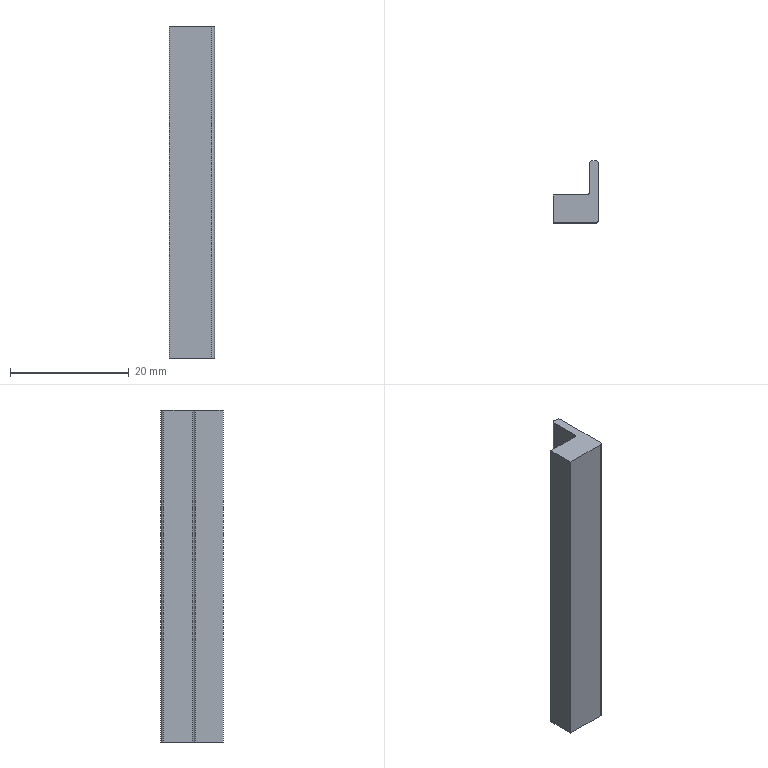Part | NX | features BREP 2 | 2 solids | 24 faces | box 7.6 x 10.5 x 56 mm | volume 4963 mm3 | plane 16 | cylinder 8 | commonest cylinder face diameters 1 x8
STEP:
#1=CARTESIAN_POINT('',(2.3,-0.05,-4.));
#2=VERTEX_POINT('',#1);
#3=CARTESIAN_POINT('',(2.3,-0.05,52.));
#4=VERTEX_POINT('',#3);
#5=CARTESIAN_POINT('',(2.3,-0.05,0.));
#6=DIRECTION('',(0.,0.,1.));
#7=VECTOR('',#6,1000.);
#8=LINE('',#5,#7);
#9=EDGE_CURVE('',#2,#4,#8,.T.);
#10=ORIENTED_EDGE('',*,*,#9,.T.);
#11=CARTESIAN_POINT('',(2.3,4.75,52.));
#12=VERTEX_POINT('',#11);
#13=CARTESIAN_POINT('',(2.3,4.728,52.));
#14=DIRECTION('',(0.,-1.,0.));
#15=VECTOR('',#14,1000.);
#16=LINE('',#13,#15);
#17=EDGE_CURVE('',#12,#4,#16,.T.);
#18=ORIENTED_EDGE('',*,*,#17,.F.);
#19=CARTESIAN_POINT('',(2.3,4.75,-4.));
#20=VERTEX_POINT('',#19);
#21=CARTESIAN_POINT('',(2.3,4.75,0.));
#22=DIRECTION('',(0.,0.,1.));
#23=VECTOR('',#22,1000.);
#24=LINE('',#21,#23);
#25=EDGE_CURVE('',#20,#12,#24,.T.);
#26=ORIENTED_EDGE('',*,*,#25,.F.);
#27=CARTESIAN_POINT('',(2.3,4.728,-4.));
#28=DIRECTION('',(0.,-1.,0.));
#29=VECTOR('',#28,1000.);
#30=LINE('',#27,#29);
#31=EDGE_CURVE('',#20,#2,#30,.T.);
#32=ORIENTED_EDGE('',*,*,#31,.T.);
#33=EDGE_LOOP('',(#10,#18,#26,#32));
#34=FACE_BOUND('',#33,.T.);
#35=CARTESIAN_POINT('',(2.3,-0.05,0.));
#36=DIRECTION('',(1.,0.,0.));
#37=DIRECTION('',(0.,-1.,0.));
#38=AXIS2_PLACEMENT_3D('',#35,#36,#37);
#39=PLANE('',#38);
#40=ADVANCED_FACE('',(#34),#39,.F.);
#41=ORIENTED_EDGE('',*,*,#25,.T.);
#42=CARTESIAN_POINT('',(2.8,5.25,52.));
#43=VERTEX_POINT('',#42);
#44=CARTESIAN_POINT('',(2.8,4.75,52.));
#45=DIRECTION('',(0.,0.,1.));
#46=DIRECTION('',(1.,0.,0.));
#47=AXIS2_PLACEMENT_3D('',#44,#45,#46);
#48=CIRCLE('',#47,0.5);
#49=EDGE_CURVE('',#43,#12,#48,.T.);
#50=ORIENTED_EDGE('',*,*,#49,.F.);
#51=CARTESIAN_POINT('',(2.8,5.25,-4.));
#52=VERTEX_POINT('',#51);
#53=CARTESIAN_POINT('',(2.8,5.25,0.));
#54=DIRECTION('',(0.,0.,1.));
#55=VECTOR('',#54,1000.);
#56=LINE('',#53,#55);
#57=EDGE_CURVE('',#52,#43,#56,.T.);
#58=ORIENTED_EDGE('',*,*,#57,.F.);
#59=CARTESIAN_POINT('',(2.8,4.75,-4.));
#60=DIRECTION('',(0.,0.,1.));
#61=DIRECTION('',(1.,0.,0.));
#62=AXIS2_PLACEMENT_3D('',#59,#60,#61);
#63=CIRCLE('',#62,0.5);
#64=EDGE_CURVE('',#52,#20,#63,.T.);
#65=ORIENTED_EDGE('',*,*,#64,.T.);
#66=EDGE_LOOP('',(#41,#50,#58,#65));
#67=FACE_BOUND('',#66,.T.);
#68=CARTESIAN_POINT('',(2.8,4.75,0.));
#69=DIRECTION('',(0.,0.,1.));
#70=DIRECTION('',(-1.,0.,0.));
#71=AXIS2_PLACEMENT_3D('',#68,#69,#70);
#72=CYLINDRICAL_SURFACE('',#71,0.5);
#73=ADVANCED_FACE('',(#67),#72,.T.);
#74=ORIENTED_EDGE('',*,*,#57,.T.);
#75=CARTESIAN_POINT('',(3.3,5.25,52.));
#76=VERTEX_POINT('',#75);
#77=CARTESIAN_POINT('',(5.273,5.25,52.));
#78=DIRECTION('',(-1.,0.,0.));
#79=VECTOR('',#78,1000.);
#80=LINE('',#77,#79);
#81=EDGE_CURVE('',#76,#43,#80,.T.);
#82=ORIENTED_EDGE('',*,*,#81,.F.);
#83=CARTESIAN_POINT('',(3.3,5.25,-4.));
#84=VERTEX_POINT('',#83);
#85=CARTESIAN_POINT('',(3.3,5.25,0.));
#86=DIRECTION('',(0.,0.,1.));
#87=VECTOR('',#86,1000.);
#88=LINE('',#85,#87);
#89=EDGE_CURVE('',#84,#76,#88,.T.);
#90=ORIENTED_EDGE('',*,*,#89,.F.);
#91=CARTESIAN_POINT('',(5.273,5.25,-4.));
#92=DIRECTION('',(-1.,0.,0.));
#93=VECTOR('',#92,1000.);
#94=LINE('',#91,#93);
#95=EDGE_CURVE('',#84,#52,#94,.T.);
#96=ORIENTED_EDGE('',*,*,#95,.T.);
#97=EDGE_LOOP('',(#74,#82,#90,#96));
#98=FACE_BOUND('',#97,.T.);
#99=CARTESIAN_POINT('',(2.8,5.25,0.));
#100=DIRECTION('',(0.,-1.,0.));
#101=DIRECTION('',(-1.,0.,0.));
#102=AXIS2_PLACEMENT_3D('',#99,#100,#101);
#103=PLANE('',#102);
#104=ADVANCED_FACE('',(#98),#103,.F.);
#105=ORIENTED_EDGE('',*,*,#89,.T.);
#106=CARTESIAN_POINT('',(3.8,4.75,52.));
#107=VERTEX_POINT('',#106);
#108=CARTESIAN_POINT('',(3.3,4.75,52.));
#109=DIRECTION('',(0.,0.,1.));
#110=DIRECTION('',(1.,0.,0.));
#111=AXIS2_PLACEMENT_3D('',#108,#109,#110);
#112=CIRCLE('',#111,0.5);
#113=EDGE_CURVE('',#107,#76,#112,.T.);
#114=ORIENTED_EDGE('',*,*,#113,.F.);
#115=CARTESIAN_POINT('',(3.8,4.75,-4.));
#116=VERTEX_POINT('',#115);
#117=CARTESIAN_POINT('',(3.8,4.75,0.));
#118=DIRECTION('',(0.,0.,1.));
#119=VECTOR('',#118,1000.);
#120=LINE('',#117,#119);
#121=EDGE_CURVE('',#116,#107,#120,.T.);
#122=ORIENTED_EDGE('',*,*,#121,.F.);
#123=CARTESIAN_POINT('',(3.3,4.75,-4.));
#124=DIRECTION('',(0.,0.,1.));
#125=DIRECTION('',(1.,0.,0.));
#126=AXIS2_PLACEMENT_3D('',#123,#124,#125);
#127=CIRCLE('',#126,0.5);
#128=EDGE_CURVE('',#116,#84,#127,.T.);
#129=ORIENTED_EDGE('',*,*,#128,.T.);
#130=EDGE_LOOP('',(#105,#114,#122,#129));
#131=FACE_BOUND('',#130,.T.);
#132=CARTESIAN_POINT('',(3.3,4.75,0.));
#133=DIRECTION('',(0.,0.,1.));
#134=DIRECTION('',(-1.,0.,0.));
#135=AXIS2_PLACEMENT_3D('',#132,#133,#134);
#136=CYLINDRICAL_SURFACE('',#135,0.5);
#137=ADVANCED_FACE('',(#131),#136,.T.);
#138=ORIENTED_EDGE('',*,*,#121,.T.);
#139=CARTESIAN_POINT('',(3.8,-4.75,52.));
#140=VERTEX_POINT('',#139);
#141=CARTESIAN_POINT('',(3.8,4.728,52.));
#142=DIRECTION('',(0.,1.,0.));
#143=VECTOR('',#142,1000.);
#144=LINE('',#141,#143);
#145=EDGE_CURVE('',#140,#107,#144,.T.);
#146=ORIENTED_EDGE('',*,*,#145,.F.);
#147=CARTESIAN_POINT('',(3.8,-4.75,-4.));
#148=VERTEX_POINT('',#147);
#149=CARTESIAN_POINT('',(3.8,-4.75,0.));
#150=DIRECTION('',(0.,0.,1.));
#151=VECTOR('',#150,1000.);
#152=LINE('',#149,#151);
#153=EDGE_CURVE('',#148,#140,#152,.T.);
#154=ORIENTED_EDGE('',*,*,#153,.F.);
#155=CARTESIAN_POINT('',(3.8,4.728,-4.));
#156=DIRECTION('',(0.,1.,0.));
#157=VECTOR('',#156,1000.);
#158=LINE('',#155,#157);
#159=EDGE_CURVE('',#148,#116,#158,.T.);
#160=ORIENTED_EDGE('',*,*,#159,.T.);
#161=EDGE_LOOP('',(#138,#146,#154,#160));
#162=FACE_BOUND('',#161,.T.);
#163=CARTESIAN_POINT('',(3.8,4.75,0.));
#164=DIRECTION('',(-1.,0.,0.));
#165=DIRECTION('',(0.,1.,0.));
#166=AXIS2_PLACEMENT_3D('',#163,#164,#165);
#167=PLANE('',#166);
#168=ADVANCED_FACE('',(#162),#167,.F.);
#169=ORIENTED_EDGE('',*,*,#153,.T.);
#170=CARTESIAN_POINT('',(3.3,-5.25,52.));
#171=VERTEX_POINT('',#170);
#172=CARTESIAN_POINT('',(3.3,-4.75,52.));
#173=DIRECTION('',(0.,0.,1.));
#174=DIRECTION('',(1.,0.,0.));
#175=AXIS2_PLACEMENT_3D('',#172,#173,#174);
#176=CIRCLE('',#175,0.5);
#177=EDGE_CURVE('',#171,#140,#176,.T.);
#178=ORIENTED_EDGE('',*,*,#177,.F.);
#179=CARTESIAN_POINT('',(3.3,-5.25,-4.));
#180=VERTEX_POINT('',#179);
#181=CARTESIAN_POINT('',(3.3,-5.25,0.));
#182=DIRECTION('',(0.,0.,1.));
#183=VECTOR('',#182,1000.);
#184=LINE('',#181,#183);
#185=EDGE_CURVE('',#180,#171,#184,.T.);
#186=ORIENTED_EDGE('',*,*,#185,.F.);
#187=CARTESIAN_POINT('',(3.3,-4.75,-4.));
#188=DIRECTION('',(0.,0.,1.));
#189=DIRECTION('',(1.,0.,0.));
#190=AXIS2_PLACEMENT_3D('',#187,#188,#189);
#191=CIRCLE('',#190,0.5);
#192=EDGE_CURVE('',#180,#148,#191,.T.);
#193=ORIENTED_EDGE('',*,*,#192,.T.);
#194=EDGE_LOOP('',(#169,#178,#186,#193));
#195=FACE_BOUND('',#194,.T.);
#196=CARTESIAN_POINT('',(3.3,-4.75,0.));
#197=DIRECTION('',(0.,0.,1.));
#198=DIRECTION('',(-1.,0.,0.));
#199=AXIS2_PLACEMENT_3D('',#196,#197,#198);
#200=CYLINDRICAL_SURFACE('',#199,0.5);
#201=ADVANCED_FACE('',(#195),#200,.T.);
#202=ORIENTED_EDGE('',*,*,#185,.T.);
#203=CARTESIAN_POINT('',(-3.8,-5.25,52.));
#204=VERTEX_POINT('',#203);
#205=CARTESIAN_POINT('',(5.273,-5.25,52.));
#206=DIRECTION('',(1.,0.,0.));
#207=VECTOR('',#206,1000.);
#208=LINE('',#205,#207);
#209=EDGE_CURVE('',#204,#171,#208,.T.);
#210=ORIENTED_EDGE('',*,*,#209,.F.);
#211=CARTESIAN_POINT('',(-3.8,-5.25,-4.));
#212=VERTEX_POINT('',#211);
#213=CARTESIAN_POINT('',(-3.8,-5.25,0.));
#214=DIRECTION('',(0.,0.,1.));
#215=VECTOR('',#214,1000.);
#216=LINE('',#213,#215);
#217=EDGE_CURVE('',#212,#204,#216,.T.);
#218=ORIENTED_EDGE('',*,*,#217,.F.);
#219=CARTESIAN_POINT('',(5.273,-5.25,-4.));
#220=DIRECTION('',(1.,0.,0.));
#221=VECTOR('',#220,1000.);
#222=LINE('',#219,#221);
#223=EDGE_CURVE('',#212,#180,#222,.T.);
#224=ORIENTED_EDGE('',*,*,#223,.T.);
#225=EDGE_LOOP('',(#202,#210,#218,#224));
#226=FACE_BOUND('',#225,.T.);
#227=CARTESIAN_POINT('',(3.3,-5.25,0.));
#228=DIRECTION('',(0.,1.,0.));
#229=DIRECTION('',(1.,0.,0.));
#230=AXIS2_PLACEMENT_3D('',#227,#228,#229);
#231=PLANE('',#230);
#232=ADVANCED_FACE('',(#226),#231,.F.);
#233=ORIENTED_EDGE('',*,*,#217,.T.);
#234=CARTESIAN_POINT('',(-3.8,-0.55,52.));
#235=VERTEX_POINT('',#234);
#236=CARTESIAN_POINT('',(-3.8,4.728,52.));
#237=DIRECTION('',(0.,-1.,0.));
#238=VECTOR('',#237,1000.);
#239=LINE('',#236,#238);
#240=EDGE_CURVE('',#235,#204,#239,.T.);
#241=ORIENTED_EDGE('',*,*,#240,.F.);
#242=CARTESIAN_POINT('',(-3.8,-0.55,-4.));
#243=VERTEX_POINT('',#242);
#244=CARTESIAN_POINT('',(-3.8,-0.55,0.));
#245=DIRECTION('',(0.,0.,1.));
#246=VECTOR('',#245,1000.);
#247=LINE('',#244,#246);
#248=EDGE_CURVE('',#243,#235,#247,.T.);
#249=ORIENTED_EDGE('',*,*,#248,.F.);
#250=CARTESIAN_POINT('',(-3.8,4.728,-4.));
#251=DIRECTION('',(0.,-1.,0.));
#252=VECTOR('',#251,1000.);
#253=LINE('',#250,#252);
#254=EDGE_CURVE('',#243,#212,#253,.T.);
#255=ORIENTED_EDGE('',*,*,#254,.T.);
#256=EDGE_LOOP('',(#233,#241,#249,#255));
#257=FACE_BOUND('',#256,.T.);
#258=CARTESIAN_POINT('',(-3.8,4.728,0.));
#259=DIRECTION('',(-1.,0.,0.));
#260=DIRECTION('',(0.,1.,0.));
#261=AXIS2_PLACEMENT_3D('',#258,#259,#260);
#262=PLANE('',#261);
#263=ADVANCED_FACE('',(#257),#262,.T.);
#264=ORIENTED_EDGE('',*,*,#248,.T.);
#265=CARTESIAN_POINT('',(1.8,-0.55,52.));
#266=VERTEX_POINT('',#265);
#267=CARTESIAN_POINT('',(5.273,-0.55,52.));
#268=DIRECTION('',(-1.,0.,0.));
#269=VECTOR('',#268,1000.);
#270=LINE('',#267,#269);
#271=EDGE_CURVE('',#266,#235,#270,.T.);
#272=ORIENTED_EDGE('',*,*,#271,.F.);
#273=CARTESIAN_POINT('',(1.8,-0.55,-4.));
#274=VERTEX_POINT('',#273);
#275=CARTESIAN_POINT('',(1.8,-0.55,0.));
#276=DIRECTION('',(0.,0.,1.));
#277=VECTOR('',#276,1000.);
#278=LINE('',#275,#277);
#279=EDGE_CURVE('',#274,#266,#278,.T.);
#280=ORIENTED_EDGE('',*,*,#279,.F.);
#281=CARTESIAN_POINT('',(5.273,-0.55,-4.));
#282=DIRECTION('',(-1.,0.,0.));
#283=VECTOR('',#282,1000.);
#284=LINE('',#281,#283);
#285=EDGE_CURVE('',#274,#243,#284,.T.);
#286=ORIENTED_EDGE('',*,*,#285,.T.);
#287=EDGE_LOOP('',(#264,#272,#280,#286));
#288=FACE_BOUND('',#287,.T.);
#289=CARTESIAN_POINT('',(-9.777,-0.55,0.));
#290=DIRECTION('',(0.,-1.,0.));
#291=DIRECTION('',(-1.,0.,0.));
#292=AXIS2_PLACEMENT_3D('',#289,#290,#291);
#293=PLANE('',#292);
#294=ADVANCED_FACE('',(#288),#293,.F.);
#295=CARTESIAN_POINT('',(1.8,-0.05,-4.));
#296=DIRECTION('',(0.,0.,-1.));
#297=DIRECTION('',(1.,0.,0.));
#298=AXIS2_PLACEMENT_3D('',#295,#296,#297);
#299=CIRCLE('',#298,0.5);
#300=EDGE_CURVE('',#2,#274,#299,.T.);
#301=ORIENTED_EDGE('',*,*,#300,.T.);
#302=ORIENTED_EDGE('',*,*,#279,.T.);
#303=CARTESIAN_POINT('',(1.8,-0.05,52.));
#304=DIRECTION('',(0.,0.,-1.));
#305=DIRECTION('',(1.,0.,0.));
#306=AXIS2_PLACEMENT_3D('',#303,#304,#305);
#307=CIRCLE('',#306,0.5);
#308=EDGE_CURVE('',#4,#266,#307,.T.);
#309=ORIENTED_EDGE('',*,*,#308,.F.);
#310=ORIENTED_EDGE('',*,*,#9,.F.);
#311=EDGE_LOOP('',(#301,#302,#309,#310));
#312=FACE_BOUND('',#311,.T.);
#313=CARTESIAN_POINT('',(1.8,-0.05,0.));
#314=DIRECTION('',(0.,0.,1.));
#315=DIRECTION('',(-1.,0.,0.));
#316=AXIS2_PLACEMENT_3D('',#313,#314,#315);
#317=CYLINDRICAL_SURFACE('',#316,0.5);
#318=ADVANCED_FACE('',(#312),#317,.F.);
#319=ORIENTED_EDGE('',*,*,#271,.T.);
#320=ORIENTED_EDGE('',*,*,#240,.T.);
#321=ORIENTED_EDGE('',*,*,#209,.T.);
#322=ORIENTED_EDGE('',*,*,#177,.T.);
#323=ORIENTED_EDGE('',*,*,#145,.T.);
#324=ORIENTED_EDGE('',*,*,#113,.T.);
#325=ORIENTED_EDGE('',*,*,#81,.T.);
#326=ORIENTED_EDGE('',*,*,#49,.T.);
#327=ORIENTED_EDGE('',*,*,#17,.T.);
#328=ORIENTED_EDGE('',*,*,#308,.T.);
#329=EDGE_LOOP('',(#319,#320,#321,#322,#323,#324,#325,#326,#327,#328));
#330=FACE_BOUND('',#329,.T.);
#331=CARTESIAN_POINT('',(5.273,4.728,52.));
#332=DIRECTION('',(0.,0.,1.));
#333=DIRECTION('',(-1.,0.,0.));
#334=AXIS2_PLACEMENT_3D('',#331,#332,#333);
#335=PLANE('',#334);
#336=ADVANCED_FACE('',(#330),#335,.T.);
#337=ORIENTED_EDGE('',*,*,#285,.F.);
#338=ORIENTED_EDGE('',*,*,#300,.F.);
#339=ORIENTED_EDGE('',*,*,#31,.F.);
#340=ORIENTED_EDGE('',*,*,#64,.F.);
#341=ORIENTED_EDGE('',*,*,#95,.F.);
#342=ORIENTED_EDGE('',*,*,#128,.F.);
#343=ORIENTED_EDGE('',*,*,#159,.F.);
#344=ORIENTED_EDGE('',*,*,#192,.F.);
#345=ORIENTED_EDGE('',*,*,#223,.F.);
#346=ORIENTED_EDGE('',*,*,#254,.F.);
#347=EDGE_LOOP('',(#337,#338,#339,#340,#341,#342,#343,#344,#345,#346));
#348=FACE_BOUND('',#347,.T.);
#349=CARTESIAN_POINT('',(5.273,4.728,-4.));
#350=DIRECTION('',(0.,0.,1.));
#351=DIRECTION('',(-1.,0.,0.));
#352=AXIS2_PLACEMENT_3D('',#349,#350,#351);
#353=PLANE('',#352);
#354=ADVANCED_FACE('',(#348),#353,.F.);
#355=CLOSED_SHELL('',(#40,#73,#104,#137,#168,#201,#232,#263,#294,#318,#336,#354));
#356=MANIFOLD_SOLID_BREP('',#355);
#357=CARTESIAN_POINT('',(2.3,-0.05,-4.));
#358=VERTEX_POINT('',#357);
#359=CARTESIAN_POINT('',(2.3,-0.05,52.));
#360=VERTEX_POINT('',#359);
#361=CARTESIAN_POINT('',(2.3,-0.05,0.));
#362=DIRECTION('',(0.,0.,1.));
#363=VECTOR('',#362,1000.);
#364=LINE('',#361,#363);
#365=EDGE_CURVE('',#358,#360,#364,.T.);
#366=ORIENTED_EDGE('',*,*,#365,.T.);
#367=CARTESIAN_POINT('',(2.3,4.75,52.));
#368=VERTEX_POINT('',#367);
#369=CARTESIAN_POINT('',(2.3,4.728,52.));
#370=DIRECTION('',(0.,-1.,0.));
#371=VECTOR('',#370,1000.);
#372=LINE('',#369,#371);
#373=EDGE_CURVE('',#368,#360,#372,.T.);
#374=ORIENTED_EDGE('',*,*,#373,.F.);
#375=CARTESIAN_POINT('',(2.3,4.75,-4.));
#376=VERTEX_POINT('',#375);
#377=CARTESIAN_POINT('',(2.3,4.75,0.));
#378=DIRECTION('',(0.,0.,1.));
#379=VECTOR('',#378,1000.);
#380=LINE('',#377,#379);
#381=EDGE_CURVE('',#376,#368,#380,.T.);
#382=ORIENTED_EDGE('',*,*,#381,.F.);
#383=CARTESIAN_POINT('',(2.3,4.728,-4.));
#384=DIRECTION('',(0.,-1.,0.));
#385=VECTOR('',#384,1000.);
#386=LINE('',#383,#385);
#387=EDGE_CURVE('',#376,#358,#386,.T.);
#388=ORIENTED_EDGE('',*,*,#387,.T.);
#389=EDGE_LOOP('',(#366,#374,#382,#388));
#390=FACE_BOUND('',#389,.T.);
#391=CARTESIAN_POINT('',(2.3,-0.05,0.));
#392=DIRECTION('',(1.,0.,0.));
#393=DIRECTION('',(0.,-1.,0.));
#394=AXIS2_PLACEMENT_3D('',#391,#392,#393);
#395=PLANE('',#394);
#396=ADVANCED_FACE('',(#390),#395,.F.);
#397=ORIENTED_EDGE('',*,*,#381,.T.);
#398=CARTESIAN_POINT('',(2.8,5.25,52.));
#399=VERTEX_POINT('',#398);
#400=CARTESIAN_POINT('',(2.8,4.75,52.));
#401=DIRECTION('',(0.,0.,1.));
#402=DIRECTION('',(1.,0.,0.));
#403=AXIS2_PLACEMENT_3D('',#400,#401,#402);
#404=CIRCLE('',#403,0.5);
#405=EDGE_CURVE('',#399,#368,#404,.T.);
#406=ORIENTED_EDGE('',*,*,#405,.F.);
#407=CARTESIAN_POINT('',(2.8,5.25,-4.));
#408=VERTEX_POINT('',#407);
#409=CARTESIAN_POINT('',(2.8,5.25,0.));
#410=DIRECTION('',(0.,0.,1.));
#411=VECTOR('',#410,1000.);
#412=LINE('',#409,#411);
#413=EDGE_CURVE('',#408,#399,#412,.T.);
#414=ORIENTED_EDGE('',*,*,#413,.F.);
#415=CARTESIAN_POINT('',(2.8,4.75,-4.));
#416=DIRECTION('',(0.,0.,1.));
#417=DIRECTION('',(1.,0.,0.));
#418=AXIS2_PLACEMENT_3D('',#415,#416,#417);
#419=CIRCLE('',#418,0.5);
#420=EDGE_CURVE('',#408,#376,#419,.T.);
#421=ORIENTED_EDGE('',*,*,#420,.T.);
#422=EDGE_LOOP('',(#397,#406,#414,#421));
#423=FACE_BOUND('',#422,.T.);
#424=CARTESIAN_POINT('',(2.8,4.75,0.));
#425=DIRECTION('',(0.,0.,1.));
#426=DIRECTION('',(-1.,0.,0.));
#427=AXIS2_PLACEMENT_3D('',#424,#425,#426);
#428=CYLINDRICAL_SURFACE('',#427,0.5);
#429=ADVANCED_FACE('',(#423),#428,.T.);
#430=ORIENTED_EDGE('',*,*,#413,.T.);
#431=CARTESIAN_POINT('',(3.3,5.25,52.));
#432=VERTEX_POINT('',#431);
#433=CARTESIAN_POINT('',(5.273,5.25,52.));
#434=DIRECTION('',(-1.,0.,0.));
#435=VECTOR('',#434,1000.);
#436=LINE('',#433,#435);
#437=EDGE_CURVE('',#432,#399,#436,.T.);
#438=ORIENTED_EDGE('',*,*,#437,.F.);
#439=CARTESIAN_POINT('',(3.3,5.25,-4.));
#440=VERTEX_POINT('',#439);
#441=CARTESIAN_POINT('',(3.3,5.25,0.));
#442=DIRECTION('',(0.,0.,1.));
#443=VECTOR('',#442,1000.);
#444=LINE('',#441,#443);
#445=EDGE_CURVE('',#440,#432,#444,.T.);
#446=ORIENTED_EDGE('',*,*,#445,.F.);
#447=CARTESIAN_POINT('',(5.273,5.25,-4.));
#448=DIRECTION('',(-1.,0.,0.));
#449=VECTOR('',#448,1000.);
#450=LINE('',#447,#449);
#451=EDGE_CURVE('',#440,#408,#450,.T.);
#452=ORIENTED_EDGE('',*,*,#451,.T.);
#453=EDGE_LOOP('',(#430,#438,#446,#452));
#454=FACE_BOUND('',#453,.T.);
#455=CARTESIAN_POINT('',(2.8,5.25,0.));
#456=DIRECTION('',(0.,-1.,0.));
#457=DIRECTION('',(-1.,0.,0.));
#458=AXIS2_PLACEMENT_3D('',#455,#456,#457);
#459=PLANE('',#458);
#460=ADVANCED_FACE('',(#454),#459,.F.);
#461=ORIENTED_EDGE('',*,*,#445,.T.);
#462=CARTESIAN_POINT('',(3.8,4.75,52.));
#463=VERTEX_POINT('',#462);
#464=CARTESIAN_POINT('',(3.3,4.75,52.));
#465=DIRECTION('',(0.,0.,1.));
#466=DIRECTION('',(1.,0.,0.));
#467=AXIS2_PLACEMENT_3D('',#464,#465,#466);
#468=CIRCLE('',#467,0.5);
#469=EDGE_CURVE('',#463,#432,#468,.T.);
#470=ORIENTED_EDGE('',*,*,#469,.F.);
#471=CARTESIAN_POINT('',(3.8,4.75,-4.));
#472=VERTEX_POINT('',#471);
#473=CARTESIAN_POINT('',(3.8,4.75,0.));
#474=DIRECTION('',(0.,0.,1.));
#475=VECTOR('',#474,1000.);
#476=LINE('',#473,#475);
#477=EDGE_CURVE('',#472,#463,#476,.T.);
#478=ORIENTED_EDGE('',*,*,#477,.F.);
#479=CARTESIAN_POINT('',(3.3,4.75,-4.));
#480=DIRECTION('',(0.,0.,1.));
#481=DIRECTION('',(1.,0.,0.));
#482=AXIS2_PLACEMENT_3D('',#479,#480,#481);
#483=CIRCLE('',#482,0.5);
#484=EDGE_CURVE('',#472,#440,#483,.T.);
#485=ORIENTED_EDGE('',*,*,#484,.T.);
#486=EDGE_LOOP('',(#461,#470,#478,#485));
#487=FACE_BOUND('',#486,.T.);
#488=CARTESIAN_POINT('',(3.3,4.75,0.));
#489=DIRECTION('',(0.,0.,1.));
#490=DIRECTION('',(-1.,0.,0.));
#491=AXIS2_PLACEMENT_3D('',#488,#489,#490);
#492=CYLINDRICAL_SURFACE('',#491,0.5);
#493=ADVANCED_FACE('',(#487),#492,.T.);
#494=ORIENTED_EDGE('',*,*,#477,.T.);
#495=CARTESIAN_POINT('',(3.8,-4.75,52.));
#496=VERTEX_POINT('',#495);
#497=CARTESIAN_POINT('',(3.8,4.728,52.));
#498=DIRECTION('',(0.,1.,0.));
#499=VECTOR('',#498,1000.);
#500=LINE('',#497,#499);
#501=EDGE_CURVE('',#496,#463,#500,.T.);
#502=ORIENTED_EDGE('',*,*,#501,.F.);
#503=CARTESIAN_POINT('',(3.8,-4.75,-4.));
#504=VERTEX_POINT('',#503);
#505=CARTESIAN_POINT('',(3.8,-4.75,0.));
#506=DIRECTION('',(0.,0.,1.));
#507=VECTOR('',#506,1000.);
#508=LINE('',#505,#507);
#509=EDGE_CURVE('',#504,#496,#508,.T.);
#510=ORIENTED_EDGE('',*,*,#509,.F.);
#511=CARTESIAN_POINT('',(3.8,4.728,-4.));
#512=DIRECTION('',(0.,1.,0.));
#513=VECTOR('',#512,1000.);
#514=LINE('',#511,#513);
#515=EDGE_CURVE('',#504,#472,#514,.T.);
#516=ORIENTED_EDGE('',*,*,#515,.T.);
#517=EDGE_LOOP('',(#494,#502,#510,#516));
#518=FACE_BOUND('',#517,.T.);
#519=CARTESIAN_POINT('',(3.8,4.75,0.));
#520=DIRECTION('',(-1.,0.,0.));
#521=DIRECTION('',(0.,1.,0.));
#522=AXIS2_PLACEMENT_3D('',#519,#520,#521);
#523=PLANE('',#522);
#524=ADVANCED_FACE('',(#518),#523,.F.);
#525=ORIENTED_EDGE('',*,*,#509,.T.);
#526=CARTESIAN_POINT('',(3.3,-5.25,52.));
#527=VERTEX_POINT('',#526);
#528=CARTESIAN_POINT('',(3.3,-4.75,52.));
#529=DIRECTION('',(0.,0.,1.));
#530=DIRECTION('',(1.,0.,0.));
#531=AXIS2_PLACEMENT_3D('',#528,#529,#530);
#532=CIRCLE('',#531,0.5);
#533=EDGE_CURVE('',#527,#496,#532,.T.);
#534=ORIENTED_EDGE('',*,*,#533,.F.);
#535=CARTESIAN_POINT('',(3.3,-5.25,-4.));
#536=VERTEX_POINT('',#535);
#537=CARTESIAN_POINT('',(3.3,-5.25,0.));
#538=DIRECTION('',(0.,0.,1.));
#539=VECTOR('',#538,1000.);
#540=LINE('',#537,#539);
#541=EDGE_CURVE('',#536,#527,#540,.T.);
#542=ORIENTED_EDGE('',*,*,#541,.F.);
#543=CARTESIAN_POINT('',(3.3,-4.75,-4.));
#544=DIRECTION('',(0.,0.,1.));
#545=DIRECTION('',(1.,0.,0.));
#546=AXIS2_PLACEMENT_3D('',#543,#544,#545);
#547=CIRCLE('',#546,0.5);
#548=EDGE_CURVE('',#536,#504,#547,.T.);
#549=ORIENTED_EDGE('',*,*,#548,.T.);
#550=EDGE_LOOP('',(#525,#534,#542,#549));
#551=FACE_BOUND('',#550,.T.);
#552=CARTESIAN_POINT('',(3.3,-4.75,0.));
#553=DIRECTION('',(0.,0.,1.));
#554=DIRECTION('',(-1.,0.,0.));
#555=AXIS2_PLACEMENT_3D('',#552,#553,#554);
#556=CYLINDRICAL_SURFACE('',#555,0.5);
#557=ADVANCED_FACE('',(#551),#556,.T.);
#558=ORIENTED_EDGE('',*,*,#541,.T.);
#559=CARTESIAN_POINT('',(-3.8,-5.25,52.));
#560=VERTEX_POINT('',#559);
#561=CARTESIAN_POINT('',(5.273,-5.25,52.));
#562=DIRECTION('',(1.,0.,0.));
#563=VECTOR('',#562,1000.);
#564=LINE('',#561,#563);
#565=EDGE_CURVE('',#560,#527,#564,.T.);
#566=ORIENTED_EDGE('',*,*,#565,.F.);
#567=CARTESIAN_POINT('',(-3.8,-5.25,-4.));
#568=VERTEX_POINT('',#567);
#569=CARTESIAN_POINT('',(-3.8,-5.25,0.));
#570=DIRECTION('',(0.,0.,1.));
#571=VECTOR('',#570,1000.);
#572=LINE('',#569,#571);
#573=EDGE_CURVE('',#568,#560,#572,.T.);
#574=ORIENTED_EDGE('',*,*,#573,.F.);
#575=CARTESIAN_POINT('',(5.273,-5.25,-4.));
#576=DIRECTION('',(1.,0.,0.));
#577=VECTOR('',#576,1000.);
#578=LINE('',#575,#577);
#579=EDGE_CURVE('',#568,#536,#578,.T.);
#580=ORIENTED_EDGE('',*,*,#579,.T.);
#581=EDGE_LOOP('',(#558,#566,#574,#580));
#582=FACE_BOUND('',#581,.T.);
#583=CARTESIAN_POINT('',(3.3,-5.25,0.));
#584=DIRECTION('',(0.,1.,0.));
#585=DIRECTION('',(1.,0.,0.));
#586=AXIS2_PLACEMENT_3D('',#583,#584,#585);
#587=PLANE('',#586);
#588=ADVANCED_FACE('',(#582),#587,.F.);
#589=ORIENTED_EDGE('',*,*,#573,.T.);
#590=CARTESIAN_POINT('',(-3.8,-0.55,52.));
#591=VERTEX_POINT('',#590);
#592=CARTESIAN_POINT('',(-3.8,4.728,52.));
#593=DIRECTION('',(0.,-1.,0.));
#594=VECTOR('',#593,1000.);
#595=LINE('',#592,#594);
#596=EDGE_CURVE('',#591,#560,#595,.T.);
#597=ORIENTED_EDGE('',*,*,#596,.F.);
#598=CARTESIAN_POINT('',(-3.8,-0.55,-4.));
#599=VERTEX_POINT('',#598);
#600=CARTESIAN_POINT('',(-3.8,-0.55,0.));
#601=DIRECTION('',(0.,0.,1.));
#602=VECTOR('',#601,1000.);
#603=LINE('',#600,#602);
#604=EDGE_CURVE('',#599,#591,#603,.T.);
#605=ORIENTED_EDGE('',*,*,#604,.F.);
#606=CARTESIAN_POINT('',(-3.8,4.728,-4.));
#607=DIRECTION('',(0.,-1.,0.));
#608=VECTOR('',#607,1000.);
#609=LINE('',#606,#608);
#610=EDGE_CURVE('',#599,#568,#609,.T.);
#611=ORIENTED_EDGE('',*,*,#610,.T.);
#612=EDGE_LOOP('',(#589,#597,#605,#611));
#613=FACE_BOUND('',#612,.T.);
#614=CARTESIAN_POINT('',(-3.8,4.728,0.));
#615=DIRECTION('',(-1.,0.,0.));
#616=DIRECTION('',(0.,1.,0.));
#617=AXIS2_PLACEMENT_3D('',#614,#615,#616);
#618=PLANE('',#617);
#619=ADVANCED_FACE('',(#613),#618,.T.);
#620=ORIENTED_EDGE('',*,*,#604,.T.);
#621=CARTESIAN_POINT('',(1.8,-0.55,52.));
#622=VERTEX_POINT('',#621);
#623=CARTESIAN_POINT('',(5.273,-0.55,52.));
#624=DIRECTION('',(-1.,0.,0.));
#625=VECTOR('',#624,1000.);
#626=LINE('',#623,#625);
#627=EDGE_CURVE('',#622,#591,#626,.T.);
#628=ORIENTED_EDGE('',*,*,#627,.F.);
#629=CARTESIAN_POINT('',(1.8,-0.55,-4.));
#630=VERTEX_POINT('',#629);
#631=CARTESIAN_POINT('',(1.8,-0.55,0.));
#632=DIRECTION('',(0.,0.,1.));
#633=VECTOR('',#632,1000.);
#634=LINE('',#631,#633);
#635=EDGE_CURVE('',#630,#622,#634,.T.);
#636=ORIENTED_EDGE('',*,*,#635,.F.);
#637=CARTESIAN_POINT('',(5.273,-0.55,-4.));
#638=DIRECTION('',(-1.,0.,0.));
#639=VECTOR('',#638,1000.);
#640=LINE('',#637,#639);
#641=EDGE_CURVE('',#630,#599,#640,.T.);
#642=ORIENTED_EDGE('',*,*,#641,.T.);
#643=EDGE_LOOP('',(#620,#628,#636,#642));
#644=FACE_BOUND('',#643,.T.);
#645=CARTESIAN_POINT('',(-9.777,-0.55,0.));
#646=DIRECTION('',(0.,-1.,0.));
#647=DIRECTION('',(-1.,0.,0.));
#648=AXIS2_PLACEMENT_3D('',#645,#646,#647);
#649=PLANE('',#648);
#650=ADVANCED_FACE('',(#644),#649,.F.);
#651=CARTESIAN_POINT('',(1.8,-0.05,-4.));
#652=DIRECTION('',(0.,0.,-1.));
#653=DIRECTION('',(1.,0.,0.));
#654=AXIS2_PLACEMENT_3D('',#651,#652,#653);
#655=CIRCLE('',#654,0.5);
#656=EDGE_CURVE('',#358,#630,#655,.T.);
#657=ORIENTED_EDGE('',*,*,#656,.T.);
#658=ORIENTED_EDGE('',*,*,#635,.T.);
#659=CARTESIAN_POINT('',(1.8,-0.05,52.));
#660=DIRECTION('',(0.,0.,-1.));
#661=DIRECTION('',(1.,0.,0.));
#662=AXIS2_PLACEMENT_3D('',#659,#660,#661);
#663=CIRCLE('',#662,0.5);
#664=EDGE_CURVE('',#360,#622,#663,.T.);
#665=ORIENTED_EDGE('',*,*,#664,.F.);
#666=ORIENTED_EDGE('',*,*,#365,.F.);
#667=EDGE_LOOP('',(#657,#658,#665,#666));
#668=FACE_BOUND('',#667,.T.);
#669=CARTESIAN_POINT('',(1.8,-0.05,0.));
#670=DIRECTION('',(0.,0.,1.));
#671=DIRECTION('',(-1.,0.,0.));
#672=AXIS2_PLACEMENT_3D('',#669,#670,#671);
#673=CYLINDRICAL_SURFACE('',#672,0.5);
#674=ADVANCED_FACE('',(#668),#673,.F.);
#675=ORIENTED_EDGE('',*,*,#627,.T.);
#676=ORIENTED_EDGE('',*,*,#596,.T.);
#677=ORIENTED_EDGE('',*,*,#565,.T.);
#678=ORIENTED_EDGE('',*,*,#533,.T.);
#679=ORIENTED_EDGE('',*,*,#501,.T.);
#680=ORIENTED_EDGE('',*,*,#469,.T.);
#681=ORIENTED_EDGE('',*,*,#437,.T.);
#682=ORIENTED_EDGE('',*,*,#405,.T.);
#683=ORIENTED_EDGE('',*,*,#373,.T.);
#684=ORIENTED_EDGE('',*,*,#664,.T.);
#685=EDGE_LOOP('',(#675,#676,#677,#678,#679,#680,#681,#682,#683,#684));
#686=FACE_BOUND('',#685,.T.);
#687=CARTESIAN_POINT('',(5.273,4.728,52.));
#688=DIRECTION('',(0.,0.,1.));
#689=DIRECTION('',(-1.,0.,0.));
#690=AXIS2_PLACEMENT_3D('',#687,#688,#689);
#691=PLANE('',#690);
#692=ADVANCED_FACE('',(#686),#691,.T.);
#693=ORIENTED_EDGE('',*,*,#641,.F.);
#694=ORIENTED_EDGE('',*,*,#656,.F.);
#695=ORIENTED_EDGE('',*,*,#387,.F.);
#696=ORIENTED_EDGE('',*,*,#420,.F.);
#697=ORIENTED_EDGE('',*,*,#451,.F.);
#698=ORIENTED_EDGE('',*,*,#484,.F.);
#699=ORIENTED_EDGE('',*,*,#515,.F.);
#700=ORIENTED_EDGE('',*,*,#548,.F.);
#701=ORIENTED_EDGE('',*,*,#579,.F.);
#702=ORIENTED_EDGE('',*,*,#610,.F.);
#703=EDGE_LOOP('',(#693,#694,#695,#696,#697,#698,#699,#700,#701,#702));
#704=FACE_BOUND('',#703,.T.);
#705=CARTESIAN_POINT('',(5.273,4.728,-4.));
#706=DIRECTION('',(0.,0.,1.));
#707=DIRECTION('',(-1.,0.,0.));
#708=AXIS2_PLACEMENT_3D('',#705,#706,#707);
#709=PLANE('',#708);
#710=ADVANCED_FACE('',(#704),#709,.F.);
#711=CLOSED_SHELL('',(#396,#429,#460,#493,#524,#557,#588,#619,#650,#674,#692,#710));
#712=MANIFOLD_SOLID_BREP('',#711);
#713=(LENGTH_UNIT()NAMED_UNIT(*)SI_UNIT(.MILLI.,.METRE.));
#714=UNCERTAINTY_MEASURE_WITH_UNIT(LENGTH_MEASURE(0.00001),#713,'','');
#715=(NAMED_UNIT(*)PLANE_ANGLE_UNIT()SI_UNIT($,.RADIAN.));
#716=(NAMED_UNIT(*)SI_UNIT($,.STERADIAN.)SOLID_ANGLE_UNIT());
#717=(GEOMETRIC_REPRESENTATION_CONTEXT(3)GLOBAL_UNCERTAINTY_ASSIGNED_CONTEXT((#714))GLOBAL_UNIT_ASSIGNED_CONTEXT((#713,#715,#716))REPRESENTATION_CONTEXT('',''));
#718=ADVANCED_BREP_SHAPE_REPRESENTATION('',(#356,#712),#717);